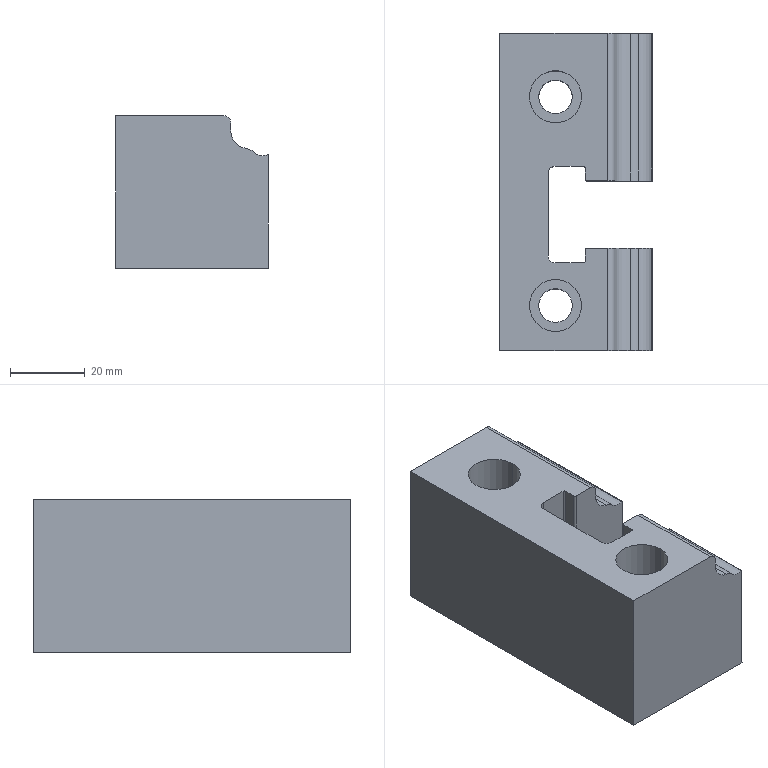Part | 1 solid | 42 faces | box 41 x 85 x 40.95 mm | volume 105466 mm3 | cylinder 24 | plane 18 | commonest cylinder face diameters 1 x4 4 x4 9 x4 14 x4 0.4 x2 6.2 x2